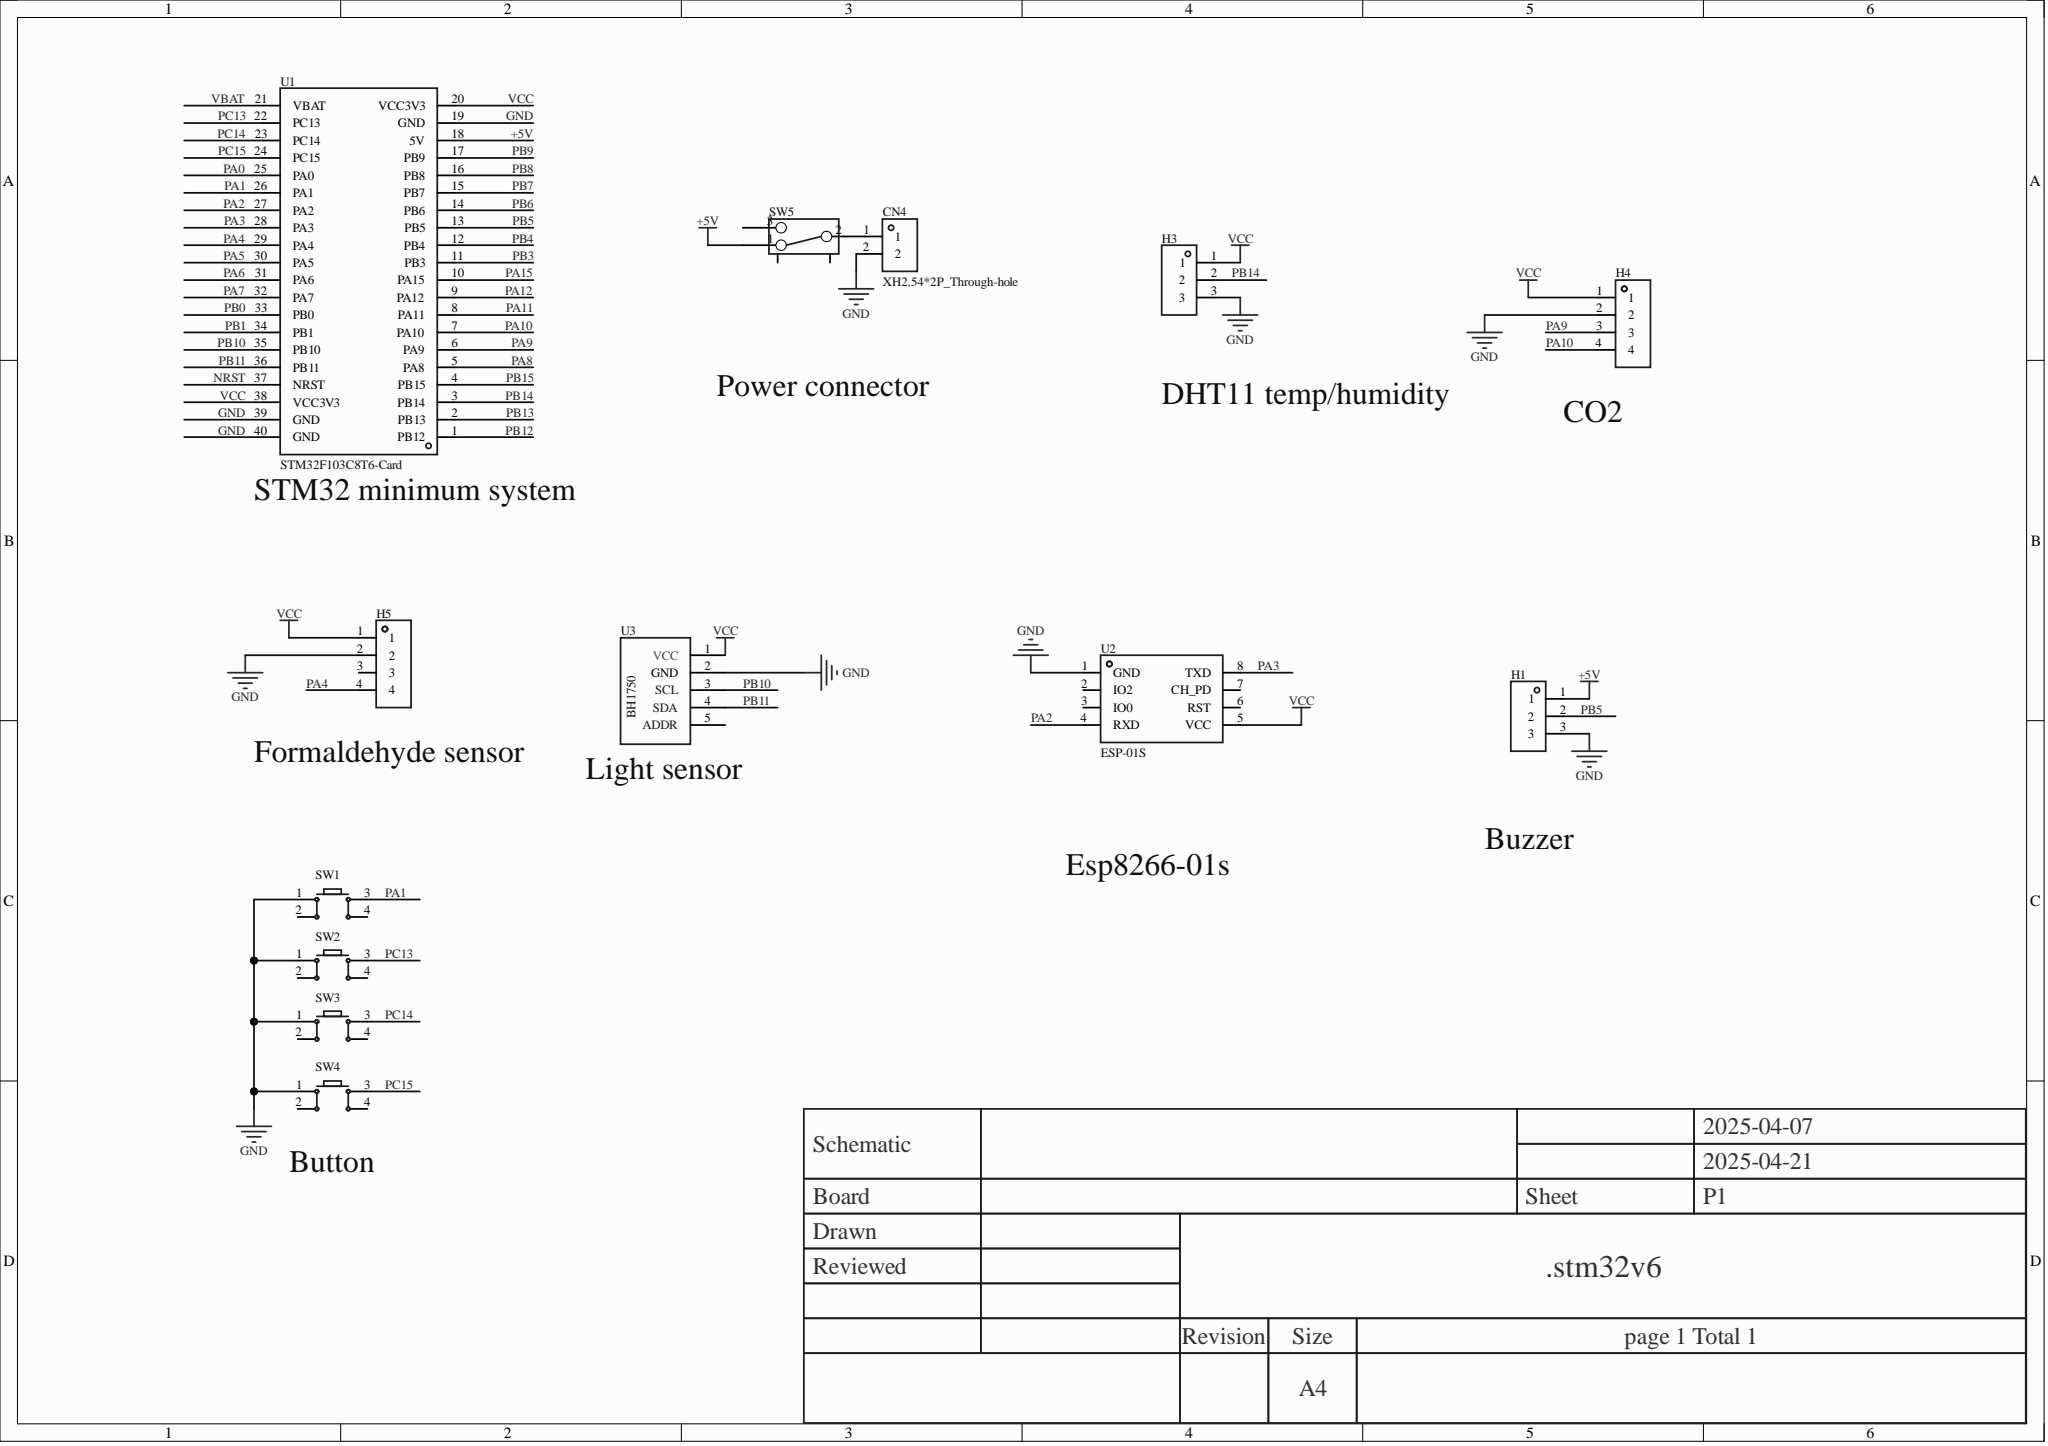Circuit board | Altium Designer | 13 parts | 17 nets
Bill of materials:
Comment,Description,Designator,Footprint,LibRef,Quantity
"XH2.54*2P_Through-hole","","CN4","CONN-TH_2P-P2.50-XH2.54-2P","XH2.54*2P_直插","1"
"","","H1, H3","HDR-TH_3P-P2.54-V-F","HDR-F_2.54_1x3P","2"
"","","H4, H5","HDR-TH_4P-P2.54-V-F","HDR-F_2.54_1x4P","2"
"","","SW1, SW2, SW3, SW4","SW-TH_4P-L6.0-W6.0-P4.50-LS6.5","Key_TH_6x6x6","4"
"","","SW5","拨动开关","拨动开关_正","1"
"STM32F103C8T6-Card","","U1","CONN-TH_L53.3-W22.9_STM32F103C8T6-CARD","STM32F103C8T6-Card","1"
"ESP-01S","","U2","WIFIM-TH_ESP-01S","ESP-01S_C111009","1"
"","","U3","BH1750光照传感器","BH1750光照传感器","1"
Netlist (Protel format):
[
CN4
CONN-TH_2P-P2.50-XH2.54-2P
XH2.54*2P_Through-hole



]
[
H1
HDR-TH_3P-P2.54-V-F




]
[
H3
HDR-TH_3P-P2.54-V-F




]
[
H4
HDR-TH_4P-P2.54-V-F




]
[
H5
HDR-TH_4P-P2.54-V-F




]
[
SW1
SW-TH_4P-L6.0-W6.0-P4.50-LS6.5




]
[
SW2
SW-TH_4P-L6.0-W6.0-P4.50-LS6.5




]
[
SW3
SW-TH_4P-L6.0-W6.0-P4.50-LS6.5




]
[
SW4
SW-TH_4P-L6.0-W6.0-P4.50-LS6.5




]
[
SW5
拨动开关




]
[
U1
CONN-TH_L53.3-W22.9_STM32F103C8T6-CARD
STM32F103C8T6-Card



]
[
U2
WIFIM-TH_ESP-01S
ESP-01S



]
[
U3
BH1750光照传感器




]
(
VCC
H3-1
H4-1
H5-1
U1-20
U1-38
U2-5
U3-1
)
(
PC15
SW4-3
U1-24
)
(
PC14
SW3-3
U1-23
)
(
PC13
SW2-3
U1-22
)
(
PB14
H3-2
U1-3
)
(
PB11
U1-36
U3-4
)
(
PB10
U1-35
U3-3
)
(
PB5
H1-2
U1-13
)
(
PA10
H4-4
U1-7
)
(
PA9
H4-3
U1-6
)
(
PA4
H5-4
U1-29
)
(
PA3
U1-28
U2-8
)
(
PA2
U1-27
U2-4
)
(
PA1
SW1-3
U1-26
)
(
NetCN4_1
CN4-1
SW5-2
)
(
GND
CN4-2
H1-3
H3-3
H4-2
H5-2
SW1-1
SW2-1
SW3-1
SW4-1
U1-19
U1-39
U1-40
U2-1
U3-2
)
(
+5V
H1-1
SW5-1
U1-18
)